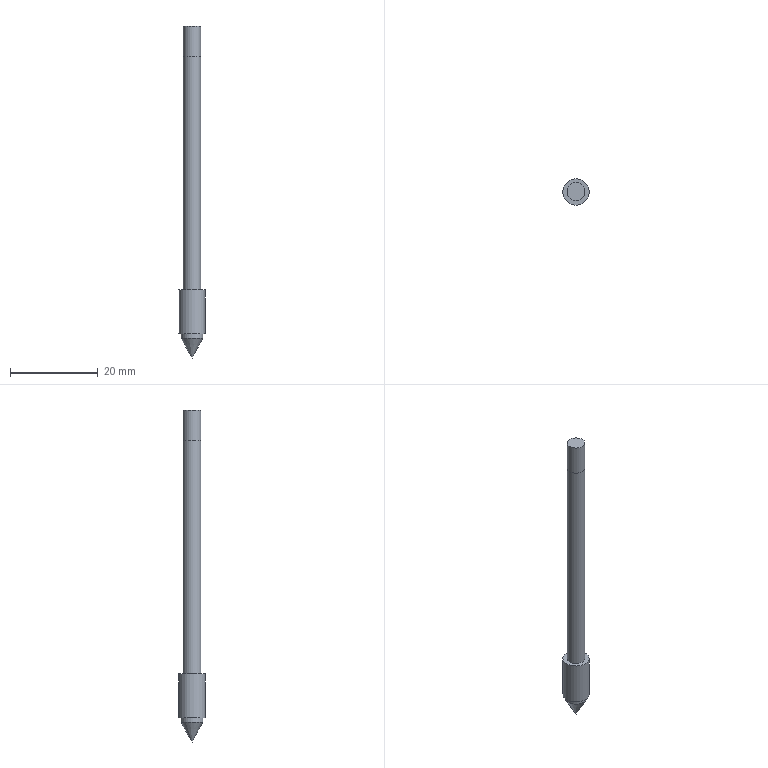Part | STEP file | 1-73.5 | 1 solid | 8 faces | box 6 x 6 x 75.5 mm | volume 1086 mm3 | cylinder 4 | plane 3 | cone 1 | commonest cylinder face diameters 4 x2 5 x1 6 x1
STEP:
#1=CARTESIAN_POINT('',(0.,0.,0.));
#2=DIRECTION('',(0.,0.,1.));
#3=DIRECTION('',(1.,0.,0.));
#4=AXIS2_PLACEMENT_3D('',#1,#2,#3);
#5=CARTESIAN_POINT('',(0.,2.,60.));
#6=VERTEX_POINT('',#5);
#7=CARTESIAN_POINT('',(0.,0.,60.));
#8=DIRECTION('',(0.,0.,1.));
#9=DIRECTION('',(0.,1.,0.));
#10=AXIS2_PLACEMENT_3D('',#7,#8,#9);
#11=CIRCLE('',#10,2.);
#12=CARTESIAN_POINT('',(0.,-0.5359,60.));
#13=DIRECTION('',(0.,0.,1.));
#14=DIRECTION('',(1.,0.,0.));
#15=AXIS2_PLACEMENT_3D('',#12,#13,#14);
#16=PLANE('',#15);
#17=CARTESIAN_POINT('',(0.,0.5359));
#18=DIRECTION('',(0.,1.));
#19=AXIS2_PLACEMENT_2D('',#17,#18);
#20=CIRCLE('',#19,2.);
#21=(GEOMETRIC_REPRESENTATION_CONTEXT(2)PARAMETRIC_REPRESENTATION_CONTEXT()REPRESENTATION_CONTEXT('',''));
#22=DEFINITIONAL_REPRESENTATION('',(#20),#21);
#23=PCURVE('',#16,#22);
#24=CARTESIAN_POINT('',(0.,0.,53.));
#25=DIRECTION('',(0.,0.,1.));
#26=DIRECTION('',(0.,1.,0.));
#27=AXIS2_PLACEMENT_3D('',#24,#25,#26);
#28=CYLINDRICAL_SURFACE('',#27,2.);
#29=CARTESIAN_POINT('',(0.,7.));
#30=DIRECTION('',(1.,0.));
#31=VECTOR('',#30,1.);
#32=LINE('',#29,#31);
#33=(GEOMETRIC_REPRESENTATION_CONTEXT(2)PARAMETRIC_REPRESENTATION_CONTEXT()REPRESENTATION_CONTEXT('',''));
#34=DEFINITIONAL_REPRESENTATION('',(#32),#33);
#35=PCURVE('',#28,#34);
#36=SURFACE_CURVE('',#11,(#23,#35),.PCURVE_S1.);
#37=EDGE_CURVE('',#6,#6,#36,.T.);
#38=ORIENTED_EDGE('',*,*,#37,.T.);
#39=EDGE_LOOP('',(#38));
#40=FACE_BOUND('',#39,.T.);
#41=ADVANCED_FACE('',(#40),#16,.T.);
#42=CARTESIAN_POINT('',(0.,3.,0.));
#43=VERTEX_POINT('',#42);
#44=CARTESIAN_POINT('',(0.,0.,0.));
#45=DIRECTION('',(0.,0.,1.));
#46=DIRECTION('',(0.,1.,0.));
#47=AXIS2_PLACEMENT_3D('',#44,#45,#46);
#48=CIRCLE('',#47,3.);
#49=CARTESIAN_POINT('',(0.,-0.8038,0.));
#50=DIRECTION('',(0.,0.,1.));
#51=DIRECTION('',(1.,0.,0.));
#52=AXIS2_PLACEMENT_3D('',#49,#50,#51);
#53=PLANE('',#52);
#54=CARTESIAN_POINT('',(0.,0.8038));
#55=DIRECTION('',(0.,1.));
#56=AXIS2_PLACEMENT_2D('',#54,#55);
#57=CIRCLE('',#56,3.);
#58=(GEOMETRIC_REPRESENTATION_CONTEXT(2)PARAMETRIC_REPRESENTATION_CONTEXT()REPRESENTATION_CONTEXT('',''));
#59=DEFINITIONAL_REPRESENTATION('',(#57),#58);
#60=PCURVE('',#53,#59);
#61=CARTESIAN_POINT('',(0.,0.,0.));
#62=DIRECTION('',(0.,0.,-1.));
#63=DIRECTION('',(0.,1.,0.));
#64=AXIS2_PLACEMENT_3D('',#61,#62,#63);
#65=CYLINDRICAL_SURFACE('',#64,3.);
#66=CARTESIAN_POINT('',(6.283,0.));
#67=DIRECTION('',(-1.,0.));
#68=VECTOR('',#67,1.);
#69=LINE('',#66,#68);
#70=(GEOMETRIC_REPRESENTATION_CONTEXT(2)PARAMETRIC_REPRESENTATION_CONTEXT()REPRESENTATION_CONTEXT('',''));
#71=DEFINITIONAL_REPRESENTATION('',(#69),#70);
#72=PCURVE('',#65,#71);
#73=SURFACE_CURVE('',#48,(#60,#72),.PCURVE_S1.);
#74=EDGE_CURVE('',#43,#43,#73,.T.);
#75=ORIENTED_EDGE('',*,*,#74,.T.);
#76=EDGE_LOOP('',(#75));
#77=FACE_BOUND('',#76,.T.);
#78=CARTESIAN_POINT('',(0.,2.,0.));
#79=VERTEX_POINT('',#78);
#80=CARTESIAN_POINT('',(0.,0.,0.));
#81=DIRECTION('',(0.,0.,1.));
#82=DIRECTION('',(0.,1.,0.));
#83=AXIS2_PLACEMENT_3D('',#80,#81,#82);
#84=CIRCLE('',#83,2.);
#85=CARTESIAN_POINT('',(0.,0.8038));
#86=DIRECTION('',(0.,1.));
#87=AXIS2_PLACEMENT_2D('',#85,#86);
#88=CIRCLE('',#87,2.);
#89=(GEOMETRIC_REPRESENTATION_CONTEXT(2)PARAMETRIC_REPRESENTATION_CONTEXT()REPRESENTATION_CONTEXT('',''));
#90=DEFINITIONAL_REPRESENTATION('',(#88),#89);
#91=PCURVE('',#53,#90);
#92=CARTESIAN_POINT('',(0.,0.,0.));
#93=DIRECTION('',(0.,0.,1.));
#94=DIRECTION('',(0.,1.,0.));
#95=AXIS2_PLACEMENT_3D('',#92,#93,#94);
#96=CYLINDRICAL_SURFACE('',#95,2.);
#97=CARTESIAN_POINT('',(0.,0.));
#98=DIRECTION('',(1.,0.));
#99=VECTOR('',#98,1.);
#100=LINE('',#97,#99);
#101=(GEOMETRIC_REPRESENTATION_CONTEXT(2)PARAMETRIC_REPRESENTATION_CONTEXT()REPRESENTATION_CONTEXT('',''));
#102=DEFINITIONAL_REPRESENTATION('',(#100),#101);
#103=PCURVE('',#96,#102);
#104=SURFACE_CURVE('',#84,(#91,#103),.PCURVE_S1.);
#105=EDGE_CURVE('',#79,#79,#104,.T.);
#106=ORIENTED_EDGE('',*,*,#105,.F.);
#107=EDGE_LOOP('',(#106));
#108=FACE_BOUND('',#107,.T.);
#109=ADVANCED_FACE('',(#77,#108),#53,.T.);
#110=CARTESIAN_POINT('',(0.,3.,-10.));
#111=VERTEX_POINT('',#110);
#112=CARTESIAN_POINT('',(0.,3.,0.));
#113=DIRECTION('',(0.,0.,-1.));
#114=VECTOR('',#113,1.);
#115=LINE('',#112,#114);
#116=CARTESIAN_POINT('',(6.283,0.));
#117=DIRECTION('',(0.,1.));
#118=VECTOR('',#117,1.);
#119=LINE('',#116,#118);
#120=(GEOMETRIC_REPRESENTATION_CONTEXT(2)PARAMETRIC_REPRESENTATION_CONTEXT()REPRESENTATION_CONTEXT('',''));
#121=DEFINITIONAL_REPRESENTATION('',(#119),#120);
#122=PCURVE('',#65,#121);
#123=CARTESIAN_POINT('',(0.,0.));
#124=DIRECTION('',(0.,1.));
#125=VECTOR('',#124,1.);
#126=LINE('',#123,#125);
#127=(GEOMETRIC_REPRESENTATION_CONTEXT(2)PARAMETRIC_REPRESENTATION_CONTEXT()REPRESENTATION_CONTEXT('',''));
#128=DEFINITIONAL_REPRESENTATION('',(#126),#127);
#129=PCURVE('',#65,#128);
#130=SEAM_CURVE('',#115,(#122,#129),.PCURVE_S1.);
#131=EDGE_CURVE('',#43,#111,#130,.T.);
#132=ORIENTED_EDGE('',*,*,#131,.T.);
#133=CARTESIAN_POINT('',(0.,0.,-10.));
#134=DIRECTION('',(0.,0.,1.));
#135=DIRECTION('',(0.,1.,0.));
#136=AXIS2_PLACEMENT_3D('',#133,#134,#135);
#137=CIRCLE('',#136,3.);
#138=CARTESIAN_POINT('',(6.283,10.));
#139=DIRECTION('',(-1.,0.));
#140=VECTOR('',#139,1.);
#141=LINE('',#138,#140);
#142=(GEOMETRIC_REPRESENTATION_CONTEXT(2)PARAMETRIC_REPRESENTATION_CONTEXT()REPRESENTATION_CONTEXT('',''));
#143=DEFINITIONAL_REPRESENTATION('',(#141),#142);
#144=PCURVE('',#65,#143);
#145=CARTESIAN_POINT('',(0.,-0.8038,-10.));
#146=DIRECTION('',(0.,0.,1.));
#147=DIRECTION('',(1.,0.,0.));
#148=AXIS2_PLACEMENT_3D('',#145,#146,#147);
#149=PLANE('',#148);
#150=CARTESIAN_POINT('',(0.,0.8038));
#151=DIRECTION('',(0.,1.));
#152=AXIS2_PLACEMENT_2D('',#150,#151);
#153=CIRCLE('',#152,3.);
#154=(GEOMETRIC_REPRESENTATION_CONTEXT(2)PARAMETRIC_REPRESENTATION_CONTEXT()REPRESENTATION_CONTEXT('',''));
#155=DEFINITIONAL_REPRESENTATION('',(#153),#154);
#156=PCURVE('',#149,#155);
#157=SURFACE_CURVE('',#137,(#144,#156),.PCURVE_S1.);
#158=EDGE_CURVE('',#111,#111,#157,.T.);
#159=ORIENTED_EDGE('',*,*,#158,.T.);
#160=ORIENTED_EDGE('',*,*,#131,.F.);
#161=ORIENTED_EDGE('',*,*,#74,.F.);
#162=EDGE_LOOP('',(#132,#159,#160,#161));
#163=FACE_BOUND('',#162,.T.);
#164=ADVANCED_FACE('',(#163),#65,.T.);
#165=ORIENTED_EDGE('',*,*,#158,.T.);
#166=EDGE_LOOP('',(#165));
#167=FACE_BOUND('',#166,.F.);
#168=CARTESIAN_POINT('',(0.,2.5,-10.));
#169=VERTEX_POINT('',#168);
#170=CARTESIAN_POINT('',(0.,0.,-10.));
#171=DIRECTION('',(0.,0.,1.));
#172=DIRECTION('',(0.,1.,0.));
#173=AXIS2_PLACEMENT_3D('',#170,#171,#172);
#174=CIRCLE('',#173,2.5);
#175=CARTESIAN_POINT('',(0.,0.8038));
#176=DIRECTION('',(0.,1.));
#177=AXIS2_PLACEMENT_2D('',#175,#176);
#178=CIRCLE('',#177,2.5);
#179=(GEOMETRIC_REPRESENTATION_CONTEXT(2)PARAMETRIC_REPRESENTATION_CONTEXT()REPRESENTATION_CONTEXT('',''));
#180=DEFINITIONAL_REPRESENTATION('',(#178),#179);
#181=PCURVE('',#149,#180);
#182=CARTESIAN_POINT('',(0.,0.,-11.));
#183=DIRECTION('',(0.,0.,1.));
#184=DIRECTION('',(0.,1.,0.));
#185=AXIS2_PLACEMENT_3D('',#182,#183,#184);
#186=CYLINDRICAL_SURFACE('',#185,2.5);
#187=CARTESIAN_POINT('',(0.,1.));
#188=DIRECTION('',(1.,0.));
#189=VECTOR('',#188,1.);
#190=LINE('',#187,#189);
#191=(GEOMETRIC_REPRESENTATION_CONTEXT(2)PARAMETRIC_REPRESENTATION_CONTEXT()REPRESENTATION_CONTEXT('',''));
#192=DEFINITIONAL_REPRESENTATION('',(#190),#191);
#193=PCURVE('',#186,#192);
#194=SURFACE_CURVE('',#174,(#181,#193),.PCURVE_S1.);
#195=EDGE_CURVE('',#169,#169,#194,.T.);
#196=ORIENTED_EDGE('',*,*,#195,.F.);
#197=EDGE_LOOP('',(#196));
#198=FACE_BOUND('',#197,.F.);
#199=ADVANCED_FACE('',(#167,#198),#149,.F.);
#200=CARTESIAN_POINT('',(0.,2.5,-11.));
#201=VERTEX_POINT('',#200);
#202=CARTESIAN_POINT('',(0.,0.,-11.));
#203=DIRECTION('',(0.,0.,1.));
#204=DIRECTION('',(0.,1.,0.));
#205=AXIS2_PLACEMENT_3D('',#202,#203,#204);
#206=CIRCLE('',#205,2.5);
#207=CARTESIAN_POINT('',(0.,0.));
#208=DIRECTION('',(1.,0.));
#209=VECTOR('',#208,1.);
#210=LINE('',#207,#209);
#211=(GEOMETRIC_REPRESENTATION_CONTEXT(2)PARAMETRIC_REPRESENTATION_CONTEXT()REPRESENTATION_CONTEXT('',''));
#212=DEFINITIONAL_REPRESENTATION('',(#210),#211);
#213=PCURVE('',#186,#212);
#214=CARTESIAN_POINT('',(0.,0.,-15.5));
#215=DIRECTION('',(0.,0.,1.));
#216=DIRECTION('',(0.,1.,0.));
#217=AXIS2_PLACEMENT_3D('',#214,#215,#216);
#218=CONICAL_SURFACE('',#217,0.,0.5071);
#219=CARTESIAN_POINT('',(0.,4.5));
#220=DIRECTION('',(1.,0.));
#221=VECTOR('',#220,1.);
#222=LINE('',#219,#221);
#223=(GEOMETRIC_REPRESENTATION_CONTEXT(2)PARAMETRIC_REPRESENTATION_CONTEXT()REPRESENTATION_CONTEXT('',''));
#224=DEFINITIONAL_REPRESENTATION('',(#222),#223);
#225=PCURVE('',#218,#224);
#226=SURFACE_CURVE('',#206,(#213,#225),.PCURVE_S1.);
#227=EDGE_CURVE('',#201,#201,#226,.T.);
#228=ORIENTED_EDGE('',*,*,#227,.T.);
#229=CARTESIAN_POINT('',(0.,2.5,-11.));
#230=DIRECTION('',(0.,0.,1.));
#231=VECTOR('',#230,1.);
#232=LINE('',#229,#231);
#233=CARTESIAN_POINT('',(6.283,0.));
#234=DIRECTION('',(0.,1.));
#235=VECTOR('',#234,1.);
#236=LINE('',#233,#235);
#237=(GEOMETRIC_REPRESENTATION_CONTEXT(2)PARAMETRIC_REPRESENTATION_CONTEXT()REPRESENTATION_CONTEXT('',''));
#238=DEFINITIONAL_REPRESENTATION('',(#236),#237);
#239=PCURVE('',#186,#238);
#240=CARTESIAN_POINT('',(0.,0.));
#241=DIRECTION('',(0.,1.));
#242=VECTOR('',#241,1.);
#243=LINE('',#240,#242);
#244=(GEOMETRIC_REPRESENTATION_CONTEXT(2)PARAMETRIC_REPRESENTATION_CONTEXT()REPRESENTATION_CONTEXT('',''));
#245=DEFINITIONAL_REPRESENTATION('',(#243),#244);
#246=PCURVE('',#186,#245);
#247=SEAM_CURVE('',#232,(#239,#246),.PCURVE_S1.);
#248=EDGE_CURVE('',#201,#169,#247,.T.);
#249=ORIENTED_EDGE('',*,*,#248,.T.);
#250=ORIENTED_EDGE('',*,*,#195,.F.);
#251=ORIENTED_EDGE('',*,*,#248,.F.);
#252=EDGE_LOOP('',(#228,#249,#250,#251));
#253=FACE_BOUND('',#252,.T.);
#254=ADVANCED_FACE('',(#253),#186,.T.);
#255=CARTESIAN_POINT('',(0.,0.,-15.5));
#256=VERTEX_POINT('',#255);
#257=CARTESIAN_POINT('',(0.,0.,-15.5));
#258=DIRECTION('',(0.,0.4856,0.8742));
#259=VECTOR('',#258,1.);
#260=LINE('',#257,#259);
#261=CARTESIAN_POINT('',(6.283,0.));
#262=DIRECTION('',(0.,1.));
#263=VECTOR('',#262,1.);
#264=LINE('',#261,#263);
#265=(GEOMETRIC_REPRESENTATION_CONTEXT(2)PARAMETRIC_REPRESENTATION_CONTEXT()REPRESENTATION_CONTEXT('',''));
#266=DEFINITIONAL_REPRESENTATION('',(#264),#265);
#267=PCURVE('',#218,#266);
#268=CARTESIAN_POINT('',(0.,0.));
#269=DIRECTION('',(0.,1.));
#270=VECTOR('',#269,1.);
#271=LINE('',#268,#270);
#272=(GEOMETRIC_REPRESENTATION_CONTEXT(2)PARAMETRIC_REPRESENTATION_CONTEXT()REPRESENTATION_CONTEXT('',''));
#273=DEFINITIONAL_REPRESENTATION('',(#271),#272);
#274=PCURVE('',#218,#273);
#275=SEAM_CURVE('',#260,(#267,#274),.PCURVE_S1.);
#276=EDGE_CURVE('',#256,#201,#275,.T.);
#277=ORIENTED_EDGE('',*,*,#276,.T.);
#278=ORIENTED_EDGE('',*,*,#227,.F.);
#279=ORIENTED_EDGE('',*,*,#276,.F.);
#280=EDGE_LOOP('',(#277,#278,#279));
#281=FACE_BOUND('',#280,.T.);
#282=ADVANCED_FACE('',(#281),#218,.T.);
#283=ORIENTED_EDGE('',*,*,#105,.T.);
#284=CARTESIAN_POINT('',(0.,2.,53.));
#285=VERTEX_POINT('',#284);
#286=CARTESIAN_POINT('',(0.,2.,0.));
#287=DIRECTION('',(0.,0.,1.));
#288=VECTOR('',#287,1.);
#289=LINE('',#286,#288);
#290=CARTESIAN_POINT('',(6.283,0.));
#291=DIRECTION('',(0.,1.));
#292=VECTOR('',#291,1.);
#293=LINE('',#290,#292);
#294=(GEOMETRIC_REPRESENTATION_CONTEXT(2)PARAMETRIC_REPRESENTATION_CONTEXT()REPRESENTATION_CONTEXT('',''));
#295=DEFINITIONAL_REPRESENTATION('',(#293),#294);
#296=PCURVE('',#96,#295);
#297=CARTESIAN_POINT('',(0.,0.));
#298=DIRECTION('',(0.,1.));
#299=VECTOR('',#298,1.);
#300=LINE('',#297,#299);
#301=(GEOMETRIC_REPRESENTATION_CONTEXT(2)PARAMETRIC_REPRESENTATION_CONTEXT()REPRESENTATION_CONTEXT('',''));
#302=DEFINITIONAL_REPRESENTATION('',(#300),#301);
#303=PCURVE('',#96,#302);
#304=SEAM_CURVE('',#289,(#296,#303),.PCURVE_S1.);
#305=EDGE_CURVE('',#79,#285,#304,.T.);
#306=ORIENTED_EDGE('',*,*,#305,.T.);
#307=CARTESIAN_POINT('',(0.,0.,53.));
#308=DIRECTION('',(0.,0.,1.));
#309=DIRECTION('',(0.,1.,0.));
#310=AXIS2_PLACEMENT_3D('',#307,#308,#309);
#311=CIRCLE('',#310,2.);
#312=CARTESIAN_POINT('',(0.,53.));
#313=DIRECTION('',(1.,0.));
#314=VECTOR('',#313,1.);
#315=LINE('',#312,#314);
#316=(GEOMETRIC_REPRESENTATION_CONTEXT(2)PARAMETRIC_REPRESENTATION_CONTEXT()REPRESENTATION_CONTEXT('',''));
#317=DEFINITIONAL_REPRESENTATION('',(#315),#316);
#318=PCURVE('',#96,#317);
#319=CARTESIAN_POINT('',(0.,0.));
#320=DIRECTION('',(1.,0.));
#321=VECTOR('',#320,1.);
#322=LINE('',#319,#321);
#323=(GEOMETRIC_REPRESENTATION_CONTEXT(2)PARAMETRIC_REPRESENTATION_CONTEXT()REPRESENTATION_CONTEXT('',''));
#324=DEFINITIONAL_REPRESENTATION('',(#322),#323);
#325=PCURVE('',#28,#324);
#326=SURFACE_CURVE('',#311,(#318,#325),.PCURVE_S1.);
#327=EDGE_CURVE('',#285,#285,#326,.T.);
#328=ORIENTED_EDGE('',*,*,#327,.F.);
#329=ORIENTED_EDGE('',*,*,#305,.F.);
#330=EDGE_LOOP('',(#283,#306,#328,#329));
#331=FACE_BOUND('',#330,.T.);
#332=ADVANCED_FACE('',(#331),#96,.T.);
#333=ORIENTED_EDGE('',*,*,#37,.F.);
#334=CARTESIAN_POINT('',(0.,2.,53.));
#335=DIRECTION('',(0.,0.,1.));
#336=VECTOR('',#335,1.);
#337=LINE('',#334,#336);
#338=CARTESIAN_POINT('',(0.,0.));
#339=DIRECTION('',(0.,1.));
#340=VECTOR('',#339,1.);
#341=LINE('',#338,#340);
#342=(GEOMETRIC_REPRESENTATION_CONTEXT(2)PARAMETRIC_REPRESENTATION_CONTEXT()REPRESENTATION_CONTEXT('',''));
#343=DEFINITIONAL_REPRESENTATION('',(#341),#342);
#344=PCURVE('',#28,#343);
#345=CARTESIAN_POINT('',(6.283,0.));
#346=DIRECTION('',(0.,1.));
#347=VECTOR('',#346,1.);
#348=LINE('',#345,#347);
#349=(GEOMETRIC_REPRESENTATION_CONTEXT(2)PARAMETRIC_REPRESENTATION_CONTEXT()REPRESENTATION_CONTEXT('',''));
#350=DEFINITIONAL_REPRESENTATION('',(#348),#349);
#351=PCURVE('',#28,#350);
#352=SEAM_CURVE('',#337,(#344,#351),.PCURVE_S1.);
#353=EDGE_CURVE('',#285,#6,#352,.T.);
#354=ORIENTED_EDGE('',*,*,#353,.F.);
#355=ORIENTED_EDGE('',*,*,#327,.T.);
#356=ORIENTED_EDGE('',*,*,#353,.T.);
#357=EDGE_LOOP('',(#333,#354,#355,#356));
#358=FACE_BOUND('',#357,.T.);
#359=ADVANCED_FACE('',(#358),#28,.T.);
#360=CLOSED_SHELL('',(#41,#109,#164,#199,#254,#282,#332,#359));
#361=MANIFOLD_SOLID_BREP('',#360);
#362=(LENGTH_UNIT()NAMED_UNIT(*)SI_UNIT(.MILLI.,.METRE.));
#363=UNCERTAINTY_MEASURE_WITH_UNIT(LENGTH_MEASURE(0.0000001),#362,'','');
#364=(NAMED_UNIT(*)PLANE_ANGLE_UNIT()SI_UNIT($,.RADIAN.));
#365=(NAMED_UNIT(*)SI_UNIT($,.STERADIAN.)SOLID_ANGLE_UNIT());
#366=(GEOMETRIC_REPRESENTATION_CONTEXT(3)GLOBAL_UNCERTAINTY_ASSIGNED_CONTEXT((#363))GLOBAL_UNIT_ASSIGNED_CONTEXT((#362,#364,#365))REPRESENTATION_CONTEXT('',''));
#367=ADVANCED_BREP_SHAPE_REPRESENTATION('',(#4,#361),#366);